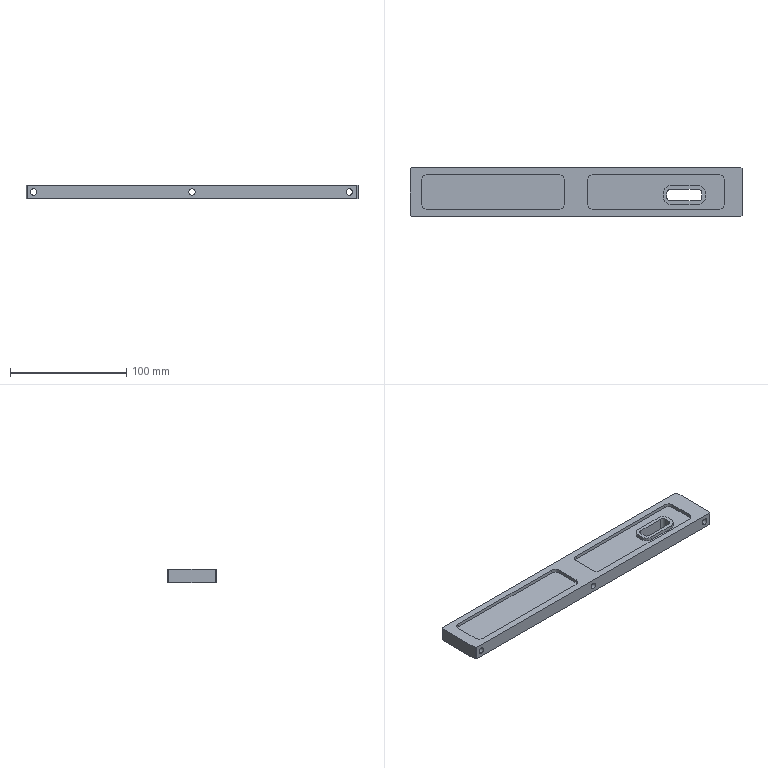Part | STEP file | J454-EBZ05-15-00-Part-1 | 1 solid | 60 faces | box 285 x 42 x 12 mm | volume 116219 mm3 | plane 32 | cylinder 28 | commonest cylinder face diameters 10 x8 5.5 x6 9.5 x6 6 x4 12 x4